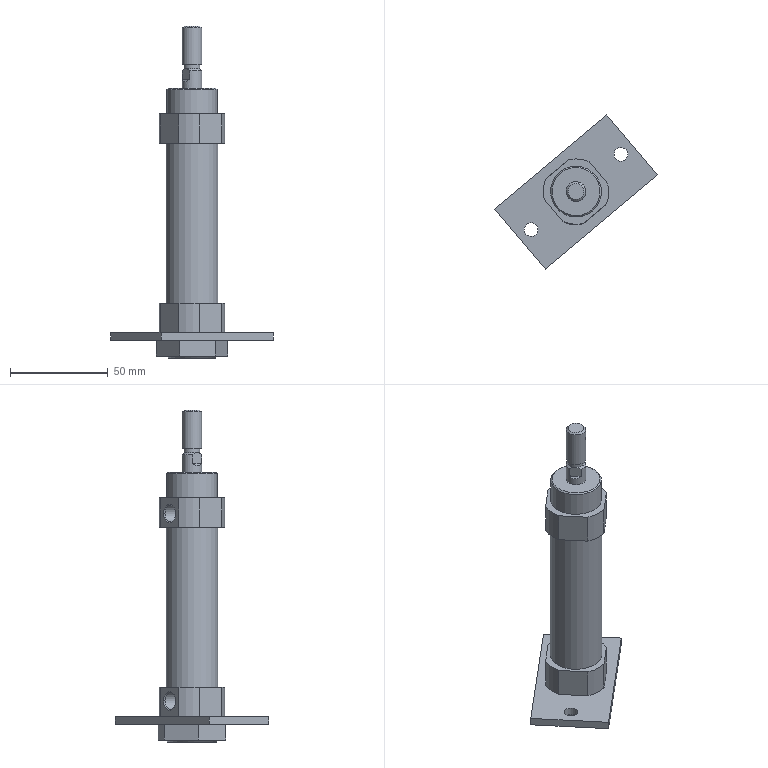Part | NX | features 1 2 | 1 solid | 61 faces | box 83.165 x 78.851 x 170 mm | volume 97303 mm3 | plane 36 | cylinder 18 | cone 7 | commonest cylinder face diameters 33.5 x8 7 x2 8.57 x2 10 x2 26 x2 8.16 x1